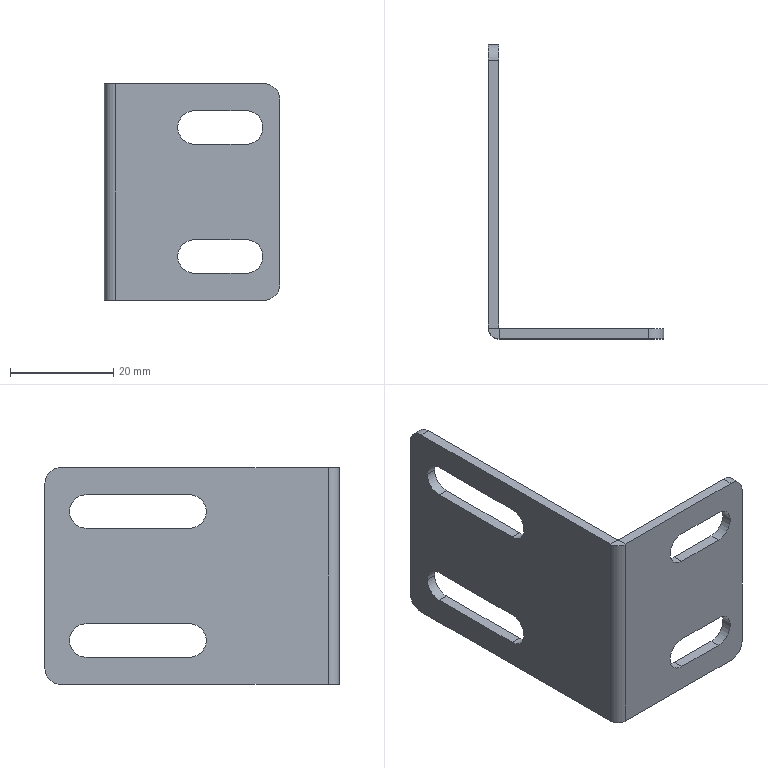Part | STEP file | Stop Mounting Plate | 1 solid | 36 faces | box 34 x 57 x 42 mm | volume 6375 mm3 | plane 20 | cylinder 16 | commonest cylinder face diameters 6.5 x10 6 x4 0.2 x1 4.2 x1